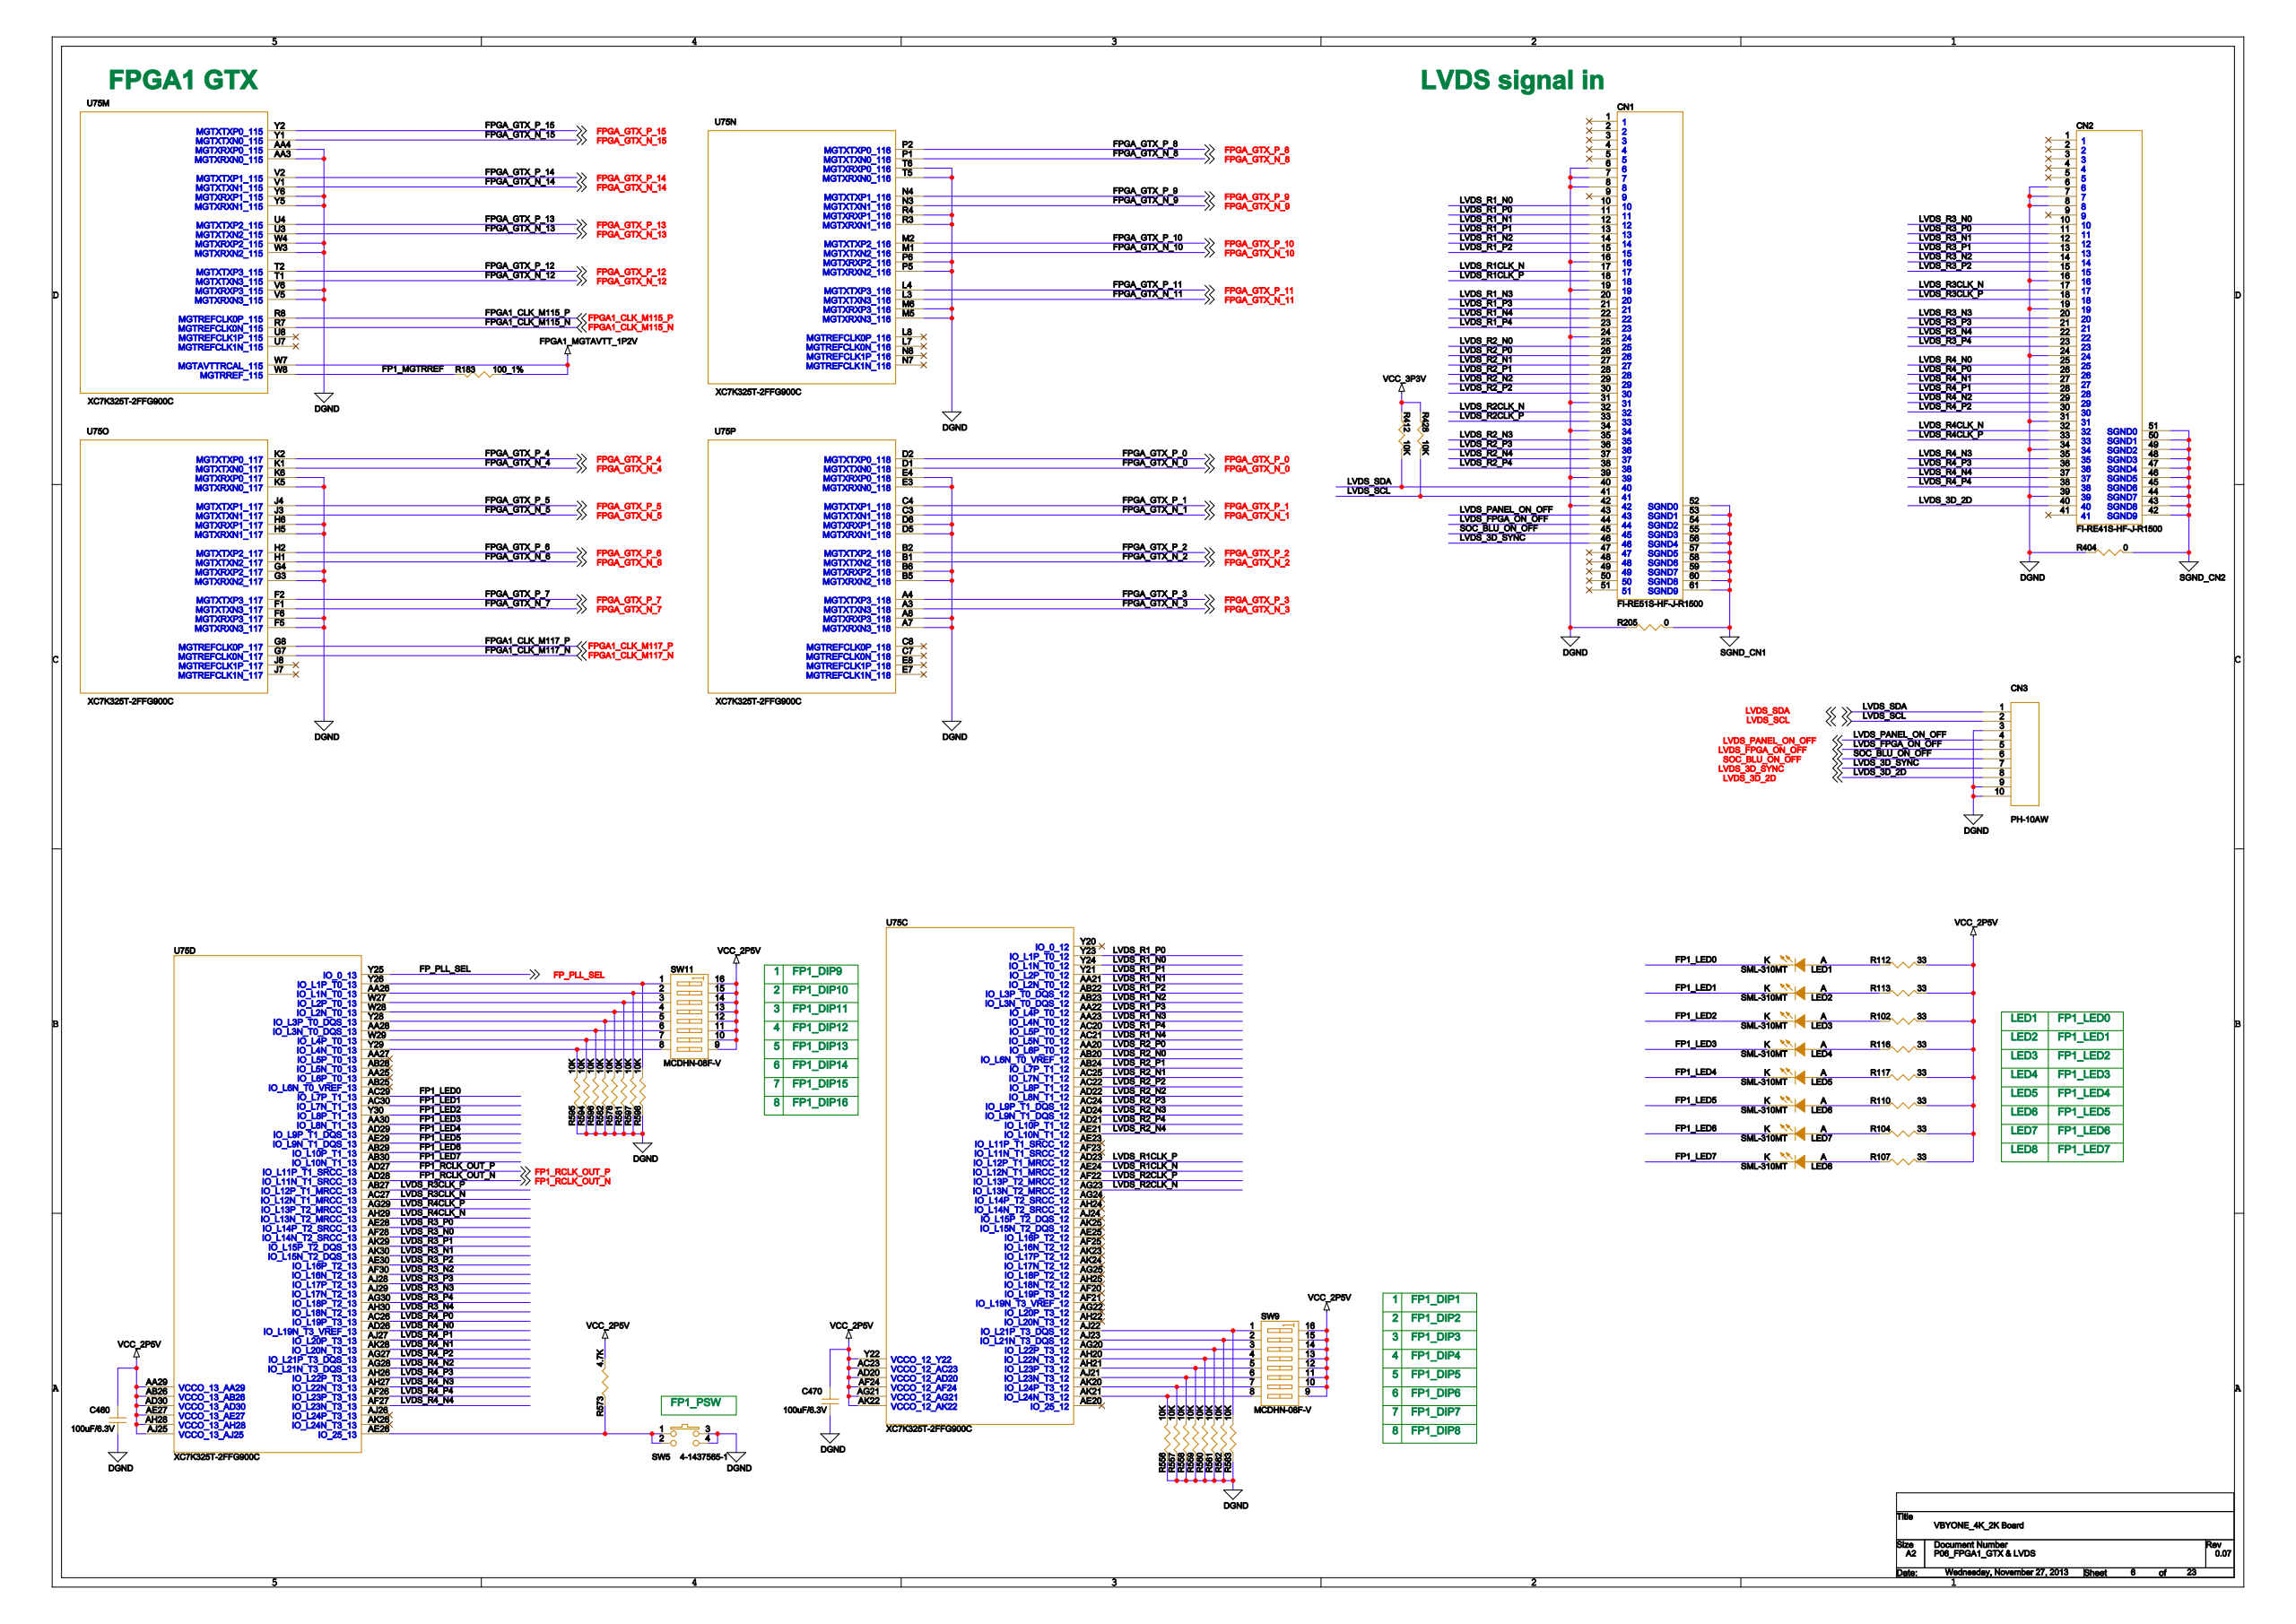Circuit board | Cadence Allegro | 1712 parts | 1495 nets | one sheet of the schematic
Parts on this sheet (reference | value | footprint):
C460 | 100uF/6.3V | CRC3225RZAS
C470 | 100uF/6.3V | CRC3225RZAS
CN1 | FI-RE51S-HF-J-R1500 | CAC051RCAS
CN2 | FI-RE41S-HF-J-R1500 | CAC041RCAS
CN3 | PH-10AW | CAD010LJAS
LED1 | SML-310MT | LEC1608RZAS
LED2 | SML-310MT | LEC1608RZAS
LED3 | SML-310MT | LEC1608RZAS
LED4 | SML-310MT | LEC1608RZAS
LED5 | SML-310MT | LEC1608RZAS
LED6 | SML-310MT | LEC1608RZAS
LED7 | SML-310MT | LEC1608RZAS
LED8 | SML-310MT | LEC1608RZAS
R102 | 33 | CRC1608RZAS
R104 | 33 | CRC1608RZAS
R107 | 33 | CRC1608RZAS
R110 | 33 | CRC1608RZAS
R112 | 33 | CRC1608RZAS
R113 | 33 | CRC1608RZAS
R116 | 33 | CRC1608RZAS
R117 | 33 | CRC1608RZAS
R183 | 100_1% | CRC1005RZAS
R205 | 0 | CRC1608RZAS
R404 | 0 | CRC1608RZAS
R412 | 10K | CRC1005RZAS
R428 | 10K | CRC1005RZAS
R556 | 10K | CRC1005RZAS
R557 | 10K | CRC1005RZAS
R558 | 10K | CRC1005RZAS
R559 | 10K | CRC1005RZAS
R560 | 10K | CRC1005RZAS
R561 | 10K | CRC1005RZAS
R562 | 10K | CRC1005RZAS
R563 | 10K | CRC1005RZAS
R573 | 4.7K | CRC1005RZAS
R578 | 10K | CRC1005RZAS
R581 | 10K | CRC1005RZAS
R582 | 10K | CRC1005RZAS
R594 | 10K | CRC1005RZAS
R595 | 10K | CRC1005RZAS
R596 | 10K | CRC1005RZAS
R597 | 10K | CRC1005RZAS
R598 | 10K | CRC1005RZAS
SW5 | 4-1437565-1 | SWC004RZBS
SW9 | MCDHN-08F-V | SWC016RHBS
SW11 | MCDHN-08F-V | SWC016RHBS
U75 | XC7K325T-2FFG900C | BGA900RGAS
Nets of these parts (net: part-pin ...):
VCC_3P3V: R412-1 R428-1
DGND: C460-1 C470-1 CN3-3 CN3-9 CN3-10 R205-1 R404-1 R556-2 R557-2 R558-2 R559-2 R560-2 R561-2 R562-2 R563-2 R578-2 R581-2 R582-2 R594-2 R595-2 R596-2 R597-2 R598-2 SW5-3 SW5-4 CN1-6 CN1-7 CN1-8 CN1-16 CN1-19 CN1-24 CN1-31 CN1-34 CN1-39 CN1-42 CN2-6 CN2-7 CN2-8 CN2-16 CN2-19 CN2-24 CN2-31 CN2-34 CN2-39 U75-A2 U75-A7 U75-A8 U75-AA3 U75-AA4 U75-B5 U75-B6 U75-D5 U75-D6 U75-E3 U75-E4 U75-F5 U75-F6 U75-G3 U75-G4 U75-H5 U75-H6 U75-K5 U75-K6 U75-M5 U75-M6 U75-P5 U75-P6 U75-R3 U75-R4 U75-T5 U75-T6 U75-V5 U75-V6 U75-W3 U75-W4 U75-Y5 U75-Y6
VCC_2P5V: C460-2 C470-2 R102-2 R104-2 R107-2 R110-2 R112-2 R113-2 R116-2 R117-2 R573-1 SW9-9 SW9-10 SW9-11 SW9-12 SW9-13 SW9-14 SW9-15 SW9-16 SW11-9 SW11-10 SW11-11 SW11-12 SW11-13 SW11-14 SW11-15 SW11-16 U75-AA29 U75-AB26 U75-AC23 U75-AD20 U75-AD30 U75-AE27 U75-AF24 U75-AG21 U75-AH28 U75-AJ25 U75-AK22 U75-Y22
FPGA1_MGTAVTT_1P2V: R183-1 U75-W7
FPGA1_CLK_M115_N: U75-R7
FPGA1_CLK_M115_P: U75-R8
FPGA1_CLK_M117_P: U75-G8
FPGA1_CLK_M117_N: U75-G7
FPGA_GTX_P_0: U75-D2
FPGA_GTX_N_0: U75-D1
FPGA_GTX_P_1: U75-C4
FPGA_GTX_N_1: U75-C3
FPGA_GTX_P_2: U75-B2
FPGA_GTX_N_2: U75-B1
FPGA_GTX_P_3: U75-A4
FPGA_GTX_N_3: U75-A3
FPGA_GTX_P_4: U75-K2
FPGA_GTX_N_4: U75-K1
FPGA_GTX_P_5: U75-J4
FPGA_GTX_N_5: U75-J3
FPGA_GTX_P_6: U75-H2
FPGA_GTX_N_6: U75-H1
FPGA_GTX_P_7: U75-F2
FPGA_GTX_N_7: U75-F1
FPGA_GTX_P_8: U75-P2
FPGA_GTX_N_8: U75-P1
FPGA_GTX_P_9: U75-N4
FPGA_GTX_N_9: U75-N3
FPGA_GTX_P_10: U75-M2
FPGA_GTX_N_10: U75-M1
FPGA_GTX_P_11: U75-L4
FPGA_GTX_N_11: U75-L3
FPGA_GTX_P_12: U75-T2
FPGA_GTX_N_12: U75-T1
FPGA_GTX_P_13: U75-U4
FPGA_GTX_N_13: U75-U3
FPGA_GTX_P_14: U75-V2
FPGA_GTX_N_14: U75-V1
FPGA_GTX_P_15: U75-Y2
FPGA_GTX_N_15: U75-Y1
FP1_RCLK_OUT_N: U75-AD28
FP1_RCLK_OUT_P: U75-AD27
SGND_CN1: R205-2 CN1-52 CN1-53 CN1-54 CN1-55 CN1-56 CN1-57 CN1-58 CN1-59 CN1-60 CN1-61
LVDS_R1_N0: CN1-10 U75-Y24
LVDS_R1_P0: CN1-11 U75-Y23
LVDS_R1_N1: CN1-12 U75-AA21
LVDS_R1_P1: CN1-13 U75-Y21
LVDS_R1_N2: CN1-14 U75-AB23
LVDS_R1_P2: CN1-15 U75-AB22
LVDS_R1CLK_N: CN1-17 U75-AE24
LVDS_R1CLK_P: CN1-18 U75-AD23
LVDS_R1_N3: CN1-20 U75-AA23
LVDS_R1_P3: CN1-21 U75-AA22
LVDS_R1_N4: CN1-22 U75-AC21
LVDS_R1_P4: CN1-23 U75-AC20
LVDS_R2_N0: CN1-25 U75-AB20
LVDS_R2_P0: CN1-26 U75-AA20
LVDS_R2_N1: CN1-27 U75-AC25
LVDS_R2_P1: CN1-28 U75-AB24
LVDS_R2_N2: CN1-29 U75-AD22
LVDS_R2_P2: CN1-30 U75-AC22
LVDS_R2CLK_N: CN1-32 U75-AG23
LVDS_R2CLK_P: CN1-33 U75-AF22
LVDS_R2_N3: CN1-35 U75-AD24
LVDS_R2_P3: CN1-36 U75-AC24
LVDS_R2_N4: CN1-37 U75-AE21
LVDS_R2_P4: CN1-38 U75-AD21
LVDS_SDA: CN3-1 R412-2 CN1-40
LVDS_SCL: CN3-2 R428-2 CN1-41
LVDS_PANEL_ON_OFF: CN3-4 CN1-43
LVDS_FPGA_ON_OFF: CN3-5 CN1-44
SOC_BLU_ON_OFF: CN3-6 CN1-45
LVDS_3D_SYNC: CN3-7 CN1-46
SGND_CN2: R404-2 CN2-42 CN2-43 CN2-44 CN2-45 CN2-46 CN2-47 CN2-48 CN2-49 CN2-50 CN2-51
LVDS_R3_N0: CN2-10 U75-AF28
LVDS_R3_P0: CN2-11 U75-AE28
LVDS_R3_N1: CN2-12 U75-AK30
LVDS_R3_P1: CN2-13 U75-AK29
LVDS_R3_N2: CN2-14 U75-AF30
LVDS_R3_P2: CN2-15 U75-AE30
LVDS_R3CLK_N: CN2-17 U75-AC27
LVDS_R3CLK_P: CN2-18 U75-AB27
LVDS_R3_N3: CN2-20 U75-AJ29
LVDS_R3_P3: CN2-21 U75-AJ28
LVDS_R3_N4: CN2-22 U75-AH30
LVDS_R3_P4: CN2-23 U75-AG30
LVDS_R4_N0: CN2-25 U75-AD26
LVDS_R4_P0: CN2-26 U75-AC26
LVDS_R4_N1: CN2-27 U75-AK28
LVDS_R4_P1: CN2-28 U75-AJ27
LVDS_R4_N2: CN2-29 U75-AG28
LVDS_R4_P2: CN2-30 U75-AG27
LVDS_R4CLK_N: CN2-32 U75-AH29
LVDS_R4CLK_P: CN2-33 U75-AG29
LVDS_R4_N3: CN2-35 U75-AH27
LVDS_R4_P3: CN2-36 U75-AH26
LVDS_R4_N4: CN2-37 U75-AF27
LVDS_R4_P4: CN2-38 U75-AF26
LVDS_3D_2D: CN3-8 CN2-40
FP_PLL_SEL: U75-Y25
N17409661: LED1-A R112-1
FP1_LED0: LED1-K U75-AC29
N17409659: LED2-A R113-1
FP1_LED1: LED2-K U75-AC30
N17409657: LED3-A R102-1
FP1_LED2: LED3-K U75-Y30
N17409655: LED4-A R116-1
FP1_LED3: LED4-K U75-AA30
N17409653: LED5-A R117-1
FP1_LED4: LED5-K U75-AD29
N19967784: LED6-A R110-1
FP1_LED5: LED6-K U75-AE29
N17409649: LED7-A R104-1
FP1_LED6: LED7-K U75-AB29
N17409647: LED8-A R107-1
FP1_LED7: LED8-K U75-AB30
FP1_MGTRREF: R183-2 U75-W8
N17474762: R573-2 SW5-1 SW5-2 U75-AE26
N19523603: R556-1 SW9-8 U75-AK21
N19523605: R557-1 SW9-7 U75-AK20
N19523627: R558-1 SW9-6 U75-AJ21
N19523629: R559-1 SW9-5 U75-AH21
N19523601: R560-1 SW9-4 U75-AH20
N19523575: R561-1 SW9-3 U75-AG20
N19523613: R562-1 SW9-2 U75-AJ23
N19523573: R563-1 SW9-1 U75-AJ22
N19498147: R578-1 SW11-4 U75-W28
N19498141: R581-1 SW11-3 U75-W27
N19498125: R582-1 SW11-5 U75-Y28
N19498151: R594-1 SW11-7 U75-W29
N19498149: R595-1 SW11-8 U75-Y29
N19498145: R596-1 SW11-6 U75-AA28
N19498143: R597-1 SW11-2 U75-AA26
N19498139: R598-1 SW11-1 U75-Y26